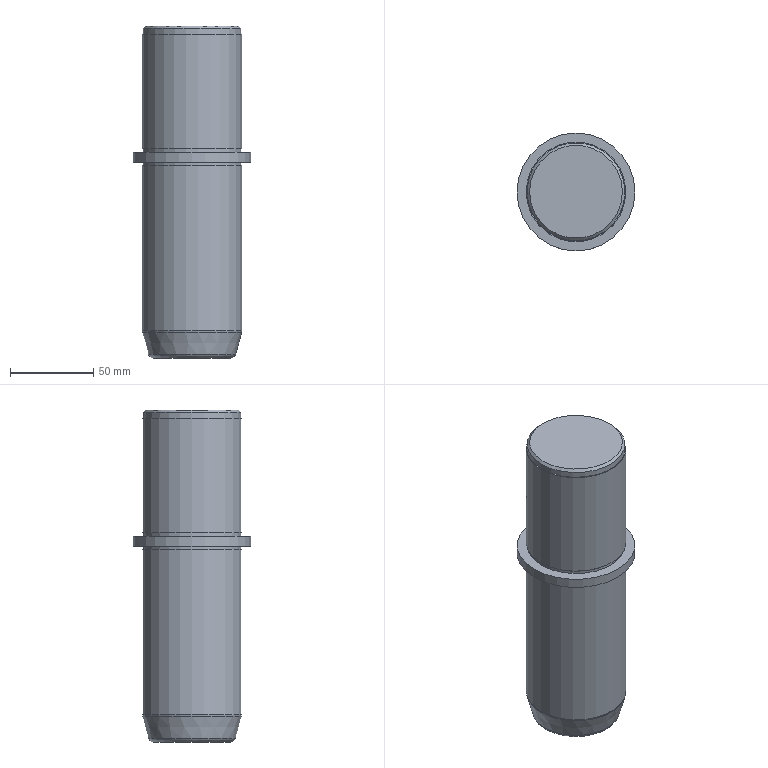Part | NX | features solid 2 | 1 solid | 17 faces | box 71 x 71 x 200 mm | volume 564911 mm3 | plane 7 | cylinder 6 | cone 2 | torus 2 | commonest cylinder face diameters 59 x3 60 x2 71 x1
STEP:
#1=CARTESIAN_POINT('',(-690.,390.,365.));
#2=VERTEX_POINT('',#1);
#3=CARTESIAN_POINT('',(-660.,390.,365.));
#4=DIRECTION('',(0.,0.,1.));
#5=DIRECTION('',(-1.,0.,0.));
#6=AXIS2_PLACEMENT_3D('',#3,#4,#5);
#7=CIRCLE('',#6,30.);
#8=EDGE_CURVE('',#2,#2,#7,.T.);
#9=ORIENTED_EDGE('',*,*,#8,.T.);
#10=EDGE_LOOP('',(#9));
#11=FACE_BOUND('',#10,.T.);
#12=CARTESIAN_POINT('',(-689.5,390.,365.));
#13=VERTEX_POINT('',#12);
#14=CARTESIAN_POINT('',(-660.,390.,365.));
#15=DIRECTION('',(0.,0.,1.));
#16=DIRECTION('',(-1.,0.,0.));
#17=AXIS2_PLACEMENT_3D('',#14,#15,#16);
#18=CIRCLE('',#17,29.5);
#19=EDGE_CURVE('',#13,#13,#18,.T.);
#20=ORIENTED_EDGE('',*,*,#19,.F.);
#21=EDGE_LOOP('',(#20));
#22=FACE_BOUND('',#21,.T.);
#23=CARTESIAN_POINT('',(-660.,390.,365.));
#24=DIRECTION('',(0.,0.,1.));
#25=DIRECTION('',(-1.,0.,0.));
#26=AXIS2_PLACEMENT_3D('',#23,#24,#25);
#27=PLANE('',#26);
#28=ADVANCED_FACE('',(#11,#22),#27,.T.);
#29=CARTESIAN_POINT('',(-689.5,390.,294.));
#30=VERTEX_POINT('',#29);
#31=CARTESIAN_POINT('',(-660.,390.,294.));
#32=DIRECTION('',(0.,0.,1.));
#33=DIRECTION('',(-1.,0.,0.));
#34=AXIS2_PLACEMENT_3D('',#31,#32,#33);
#35=CIRCLE('',#34,29.5);
#36=EDGE_CURVE('',#30,#30,#35,.F.);
#37=ORIENTED_EDGE('',*,*,#36,.F.);
#38=EDGE_LOOP('',(#37));
#39=FACE_BOUND('',#38,.T.);
#40=CARTESIAN_POINT('',(-689.5,390.,296.));
#41=VERTEX_POINT('',#40);
#42=CARTESIAN_POINT('',(-660.,390.,296.));
#43=DIRECTION('',(0.,0.,1.));
#44=DIRECTION('',(-1.,0.,0.));
#45=AXIS2_PLACEMENT_3D('',#42,#43,#44);
#46=CIRCLE('',#45,29.5);
#47=EDGE_CURVE('',#41,#41,#46,.T.);
#48=ORIENTED_EDGE('',*,*,#47,.F.);
#49=EDGE_LOOP('',(#48));
#50=FACE_BOUND('',#49,.T.);
#51=CARTESIAN_POINT('',(-660.,390.,286.));
#52=DIRECTION('',(0.,0.,1.));
#53=DIRECTION('',(-1.,0.,0.));
#54=AXIS2_PLACEMENT_3D('',#51,#52,#53);
#55=CYLINDRICAL_SURFACE('',#54,29.5);
#56=ADVANCED_FACE('',(#39,#50),#55,.T.);
#57=ORIENTED_EDGE('',*,*,#8,.F.);
#58=EDGE_LOOP('',(#57));
#59=FACE_BOUND('',#58,.T.);
#60=CARTESIAN_POINT('',(-690.,390.,296.));
#61=VERTEX_POINT('',#60);
#62=CARTESIAN_POINT('',(-660.,390.,296.));
#63=DIRECTION('',(0.,0.,1.));
#64=DIRECTION('',(-1.,0.,0.));
#65=AXIS2_PLACEMENT_3D('',#62,#63,#64);
#66=CIRCLE('',#65,30.);
#67=EDGE_CURVE('',#61,#61,#66,.T.);
#68=ORIENTED_EDGE('',*,*,#67,.T.);
#69=EDGE_LOOP('',(#68));
#70=FACE_BOUND('',#69,.T.);
#71=CARTESIAN_POINT('',(-660.,390.,365.));
#72=DIRECTION('',(0.,0.,-1.));
#73=DIRECTION('',(1.,0.,0.));
#74=AXIS2_PLACEMENT_3D('',#71,#72,#73);
#75=CYLINDRICAL_SURFACE('',#74,30.);
#76=ADVANCED_FACE('',(#59,#70),#75,.T.);
#77=ORIENTED_EDGE('',*,*,#47,.T.);
#78=EDGE_LOOP('',(#77));
#79=FACE_BOUND('',#78,.T.);
#80=ORIENTED_EDGE('',*,*,#67,.F.);
#81=EDGE_LOOP('',(#80));
#82=FACE_BOUND('',#81,.T.);
#83=CARTESIAN_POINT('',(-660.,390.,296.));
#84=DIRECTION('',(0.,0.,1.));
#85=DIRECTION('',(-1.,0.,0.));
#86=AXIS2_PLACEMENT_3D('',#83,#84,#85);
#87=PLANE('',#86);
#88=ADVANCED_FACE('',(#79,#82),#87,.F.);
#89=CARTESIAN_POINT('',(-689.5,390.,368.5));
#90=VERTEX_POINT('',#89);
#91=CARTESIAN_POINT('',(-660.,390.,368.5));
#92=DIRECTION('',(0.,0.,1.));
#93=DIRECTION('',(-1.,0.,0.));
#94=AXIS2_PLACEMENT_3D('',#91,#92,#93);
#95=CIRCLE('',#94,29.5);
#96=EDGE_CURVE('',#90,#90,#95,.F.);
#97=ORIENTED_EDGE('',*,*,#96,.T.);
#98=EDGE_LOOP('',(#97));
#99=FACE_BOUND('',#98,.T.);
#100=ORIENTED_EDGE('',*,*,#19,.T.);
#101=EDGE_LOOP('',(#100));
#102=FACE_BOUND('',#101,.T.);
#103=CARTESIAN_POINT('',(-660.,390.,370.));
#104=DIRECTION('',(0.,0.,-1.));
#105=DIRECTION('',(1.,0.,0.));
#106=AXIS2_PLACEMENT_3D('',#103,#104,#105);
#107=CYLINDRICAL_SURFACE('',#106,29.5);
#108=ADVANCED_FACE('',(#99,#102),#107,.T.);
#109=CARTESIAN_POINT('',(-688.,390.,370.));
#110=VERTEX_POINT('',#109);
#111=CARTESIAN_POINT('',(-660.,390.,370.));
#112=DIRECTION('',(0.,0.,1.));
#113=DIRECTION('',(-1.,0.,0.));
#114=AXIS2_PLACEMENT_3D('',#111,#112,#113);
#115=CIRCLE('',#114,28.);
#116=EDGE_CURVE('',#110,#110,#115,.T.);
#117=ORIENTED_EDGE('',*,*,#116,.T.);
#118=EDGE_LOOP('',(#117));
#119=FACE_BOUND('',#118,.T.);
#120=CARTESIAN_POINT('',(-660.,390.,370.));
#121=DIRECTION('',(0.,0.,1.));
#122=DIRECTION('',(-1.,0.,0.));
#123=AXIS2_PLACEMENT_3D('',#120,#121,#122);
#124=PLANE('',#123);
#125=ADVANCED_FACE('',(#119),#124,.T.);
#126=CARTESIAN_POINT('',(-695.5,390.,288.));
#127=VERTEX_POINT('',#126);
#128=CARTESIAN_POINT('',(-660.,390.,288.));
#129=DIRECTION('',(0.,0.,1.));
#130=DIRECTION('',(-1.,0.,0.));
#131=AXIS2_PLACEMENT_3D('',#128,#129,#130);
#132=CIRCLE('',#131,35.5);
#133=EDGE_CURVE('',#127,#127,#132,.T.);
#134=ORIENTED_EDGE('',*,*,#133,.T.);
#135=EDGE_LOOP('',(#134));
#136=FACE_BOUND('',#135,.T.);
#137=CARTESIAN_POINT('',(-695.5,390.,294.));
#138=VERTEX_POINT('',#137);
#139=CARTESIAN_POINT('',(-660.,390.,294.));
#140=DIRECTION('',(0.,0.,1.));
#141=DIRECTION('',(-1.,0.,0.));
#142=AXIS2_PLACEMENT_3D('',#139,#140,#141);
#143=CIRCLE('',#142,35.5);
#144=EDGE_CURVE('',#138,#138,#143,.T.);
#145=ORIENTED_EDGE('',*,*,#144,.F.);
#146=EDGE_LOOP('',(#145));
#147=FACE_BOUND('',#146,.T.);
#148=CARTESIAN_POINT('',(-660.,390.,288.));
#149=DIRECTION('',(0.,0.,1.));
#150=DIRECTION('',(-1.,0.,0.));
#151=AXIS2_PLACEMENT_3D('',#148,#149,#150);
#152=CYLINDRICAL_SURFACE('',#151,35.5);
#153=ADVANCED_FACE('',(#136,#147),#152,.T.);
#154=CARTESIAN_POINT('',(-689.5,390.,288.));
#155=VERTEX_POINT('',#154);
#156=CARTESIAN_POINT('',(-660.,390.,288.));
#157=DIRECTION('',(0.,0.,1.));
#158=DIRECTION('',(-1.,0.,0.));
#159=AXIS2_PLACEMENT_3D('',#156,#157,#158);
#160=CIRCLE('',#159,29.5);
#161=EDGE_CURVE('',#155,#155,#160,.F.);
#162=ORIENTED_EDGE('',*,*,#161,.F.);
#163=EDGE_LOOP('',(#162));
#164=FACE_BOUND('',#163,.T.);
#165=ORIENTED_EDGE('',*,*,#133,.F.);
#166=EDGE_LOOP('',(#165));
#167=FACE_BOUND('',#166,.T.);
#168=CARTESIAN_POINT('',(-660.,390.,288.));
#169=DIRECTION('',(0.,0.,1.));
#170=DIRECTION('',(-1.,0.,0.));
#171=AXIS2_PLACEMENT_3D('',#168,#169,#170);
#172=PLANE('',#171);
#173=ADVANCED_FACE('',(#164,#167),#172,.F.);
#174=ORIENTED_EDGE('',*,*,#36,.T.);
#175=EDGE_LOOP('',(#174));
#176=FACE_BOUND('',#175,.T.);
#177=ORIENTED_EDGE('',*,*,#144,.T.);
#178=EDGE_LOOP('',(#177));
#179=FACE_BOUND('',#178,.T.);
#180=CARTESIAN_POINT('',(-660.,390.,294.));
#181=DIRECTION('',(0.,0.,1.));
#182=DIRECTION('',(-1.,0.,0.));
#183=AXIS2_PLACEMENT_3D('',#180,#181,#182);
#184=PLANE('',#183);
#185=ADVANCED_FACE('',(#176,#179),#184,.T.);
#186=CARTESIAN_POINT('',(-683.411,390.,170.));
#187=VERTEX_POINT('',#186);
#188=CARTESIAN_POINT('',(-660.,390.,170.));
#189=DIRECTION('',(0.,0.,1.));
#190=DIRECTION('',(-1.,0.,0.));
#191=AXIS2_PLACEMENT_3D('',#188,#189,#190);
#192=CIRCLE('',#191,23.411);
#193=EDGE_CURVE('',#187,#187,#192,.F.);
#194=ORIENTED_EDGE('',*,*,#193,.T.);
#195=EDGE_LOOP('',(#194));
#196=FACE_BOUND('',#195,.T.);
#197=CARTESIAN_POINT('',(-660.,390.,170.));
#198=DIRECTION('',(0.,0.,1.));
#199=DIRECTION('',(-1.,0.,0.));
#200=AXIS2_PLACEMENT_3D('',#197,#198,#199);
#201=PLANE('',#200);
#202=ADVANCED_FACE('',(#196),#201,.F.);
#203=CARTESIAN_POINT('',(-630.102,390.,185.619));
#204=VERTEX_POINT('',#203);
#205=CARTESIAN_POINT('',(-660.,390.,185.619));
#206=DIRECTION('',(0.,0.,-1.));
#207=DIRECTION('',(1.,0.,0.));
#208=AXIS2_PLACEMENT_3D('',#205,#206,#207);
#209=CIRCLE('',#208,29.898);
#210=EDGE_CURVE('',#204,#204,#209,.T.);
#211=ORIENTED_EDGE('',*,*,#210,.T.);
#212=EDGE_LOOP('',(#211));
#213=FACE_BOUND('',#212,.T.);
#214=CARTESIAN_POINT('',(-686.309,390.,172.224));
#215=VERTEX_POINT('',#214);
#216=CARTESIAN_POINT('',(-660.,390.,172.224));
#217=DIRECTION('',(0.,0.,1.));
#218=DIRECTION('',(-1.,0.,0.));
#219=AXIS2_PLACEMENT_3D('',#216,#217,#218);
#220=CIRCLE('',#219,26.309);
#221=EDGE_CURVE('',#215,#215,#220,.T.);
#222=ORIENTED_EDGE('',*,*,#221,.T.);
#223=EDGE_LOOP('',(#222));
#224=FACE_BOUND('',#223,.T.);
#225=CARTESIAN_POINT('',(-660.,390.,186.));
#226=DIRECTION('',(0.,0.,1.));
#227=DIRECTION('',(1.,0.,0.));
#228=AXIS2_PLACEMENT_3D('',#225,#226,#227);
#229=CONICAL_SURFACE('',#228,30.,0.2618);
#230=ADVANCED_FACE('',(#213,#224),#229,.T.);
#231=CARTESIAN_POINT('',(-630.,390.,186.395));
#232=VERTEX_POINT('',#231);
#233=CARTESIAN_POINT('',(-660.,390.,186.395));
#234=DIRECTION('',(0.,0.,-1.));
#235=DIRECTION('',(1.,0.,0.));
#236=AXIS2_PLACEMENT_3D('',#233,#234,#235);
#237=CIRCLE('',#236,30.);
#238=EDGE_CURVE('',#232,#232,#237,.F.);
#239=ORIENTED_EDGE('',*,*,#238,.T.);
#240=EDGE_LOOP('',(#239));
#241=FACE_BOUND('',#240,.T.);
#242=CARTESIAN_POINT('',(-690.,390.,286.));
#243=VERTEX_POINT('',#242);
#244=CARTESIAN_POINT('',(-660.,390.,286.));
#245=DIRECTION('',(0.,0.,1.));
#246=DIRECTION('',(-1.,0.,0.));
#247=AXIS2_PLACEMENT_3D('',#244,#245,#246);
#248=CIRCLE('',#247,30.);
#249=EDGE_CURVE('',#243,#243,#248,.T.);
#250=ORIENTED_EDGE('',*,*,#249,.F.);
#251=EDGE_LOOP('',(#250));
#252=FACE_BOUND('',#251,.T.);
#253=CARTESIAN_POINT('',(-660.,390.,136.));
#254=DIRECTION('',(0.,0.,1.));
#255=DIRECTION('',(-1.,0.,0.));
#256=AXIS2_PLACEMENT_3D('',#253,#254,#255);
#257=CYLINDRICAL_SURFACE('',#256,30.);
#258=ADVANCED_FACE('',(#241,#252),#257,.T.);
#259=CARTESIAN_POINT('',(-689.5,390.,286.));
#260=VERTEX_POINT('',#259);
#261=CARTESIAN_POINT('',(-660.,390.,286.));
#262=DIRECTION('',(0.,0.,1.));
#263=DIRECTION('',(-1.,0.,0.));
#264=AXIS2_PLACEMENT_3D('',#261,#262,#263);
#265=CIRCLE('',#264,29.5);
#266=EDGE_CURVE('',#260,#260,#265,.T.);
#267=ORIENTED_EDGE('',*,*,#266,.F.);
#268=EDGE_LOOP('',(#267));
#269=FACE_BOUND('',#268,.T.);
#270=ORIENTED_EDGE('',*,*,#249,.T.);
#271=EDGE_LOOP('',(#270));
#272=FACE_BOUND('',#271,.T.);
#273=CARTESIAN_POINT('',(-660.,390.,286.));
#274=DIRECTION('',(0.,0.,1.));
#275=DIRECTION('',(-1.,0.,0.));
#276=AXIS2_PLACEMENT_3D('',#273,#274,#275);
#277=PLANE('',#276);
#278=ADVANCED_FACE('',(#269,#272),#277,.T.);
#279=ORIENTED_EDGE('',*,*,#266,.T.);
#280=EDGE_LOOP('',(#279));
#281=FACE_BOUND('',#280,.T.);
#282=ORIENTED_EDGE('',*,*,#161,.T.);
#283=EDGE_LOOP('',(#282));
#284=FACE_BOUND('',#283,.T.);
#285=CARTESIAN_POINT('',(-660.,390.,286.));
#286=DIRECTION('',(0.,0.,1.));
#287=DIRECTION('',(-1.,0.,0.));
#288=AXIS2_PLACEMENT_3D('',#285,#286,#287);
#289=CYLINDRICAL_SURFACE('',#288,29.5);
#290=ADVANCED_FACE('',(#281,#284),#289,.T.);
#291=ORIENTED_EDGE('',*,*,#96,.F.);
#292=EDGE_LOOP('',(#291));
#293=FACE_BOUND('',#292,.T.);
#294=ORIENTED_EDGE('',*,*,#116,.F.);
#295=EDGE_LOOP('',(#294));
#296=FACE_BOUND('',#295,.T.);
#297=CARTESIAN_POINT('',(-660.,390.,370.));
#298=DIRECTION('',(0.,0.,-1.));
#299=DIRECTION('',(1.,0.,0.));
#300=AXIS2_PLACEMENT_3D('',#297,#298,#299);
#301=CONICAL_SURFACE('',#300,28.,0.7854);
#302=ADVANCED_FACE('',(#293,#296),#301,.T.);
#303=ORIENTED_EDGE('',*,*,#210,.F.);
#304=EDGE_LOOP('',(#303));
#305=FACE_BOUND('',#304,.T.);
#306=ORIENTED_EDGE('',*,*,#238,.F.);
#307=EDGE_LOOP('',(#306));
#308=FACE_BOUND('',#307,.T.);
#309=CARTESIAN_POINT('',(-660.,390.,186.395));
#310=DIRECTION('',(0.,0.,-1.));
#311=DIRECTION('',(1.,0.,0.));
#312=AXIS2_PLACEMENT_3D('',#309,#310,#311);
#313=TOROIDAL_SURFACE('',#312,27.,3.);
#314=ADVANCED_FACE('',(#305,#308),#313,.T.);
#315=ORIENTED_EDGE('',*,*,#193,.F.);
#316=EDGE_LOOP('',(#315));
#317=FACE_BOUND('',#316,.T.);
#318=ORIENTED_EDGE('',*,*,#221,.F.);
#319=EDGE_LOOP('',(#318));
#320=FACE_BOUND('',#319,.T.);
#321=CARTESIAN_POINT('',(-660.,390.,173.));
#322=DIRECTION('',(0.,0.,1.));
#323=DIRECTION('',(-1.,0.,0.));
#324=AXIS2_PLACEMENT_3D('',#321,#322,#323);
#325=TOROIDAL_SURFACE('',#324,23.411,3.);
#326=ADVANCED_FACE('',(#317,#320),#325,.T.);
#327=CLOSED_SHELL('',(#28,#56,#76,#88,#108,#125,#153,#173,#185,#202,#230,#258,#278,#290,#302,#314,#326));
#328=MANIFOLD_SOLID_BREP('',#327);
#329=(LENGTH_UNIT()NAMED_UNIT(*)SI_UNIT(.MILLI.,.METRE.));
#330=UNCERTAINTY_MEASURE_WITH_UNIT(LENGTH_MEASURE(0.00001),#329,'','');
#331=(NAMED_UNIT(*)PLANE_ANGLE_UNIT()SI_UNIT($,.RADIAN.));
#332=(NAMED_UNIT(*)SI_UNIT($,.STERADIAN.)SOLID_ANGLE_UNIT());
#333=(GEOMETRIC_REPRESENTATION_CONTEXT(3)GLOBAL_UNCERTAINTY_ASSIGNED_CONTEXT((#330))GLOBAL_UNIT_ASSIGNED_CONTEXT((#329,#331,#332))REPRESENTATION_CONTEXT('',''));
#334=ADVANCED_BREP_SHAPE_REPRESENTATION('',(#328),#333);